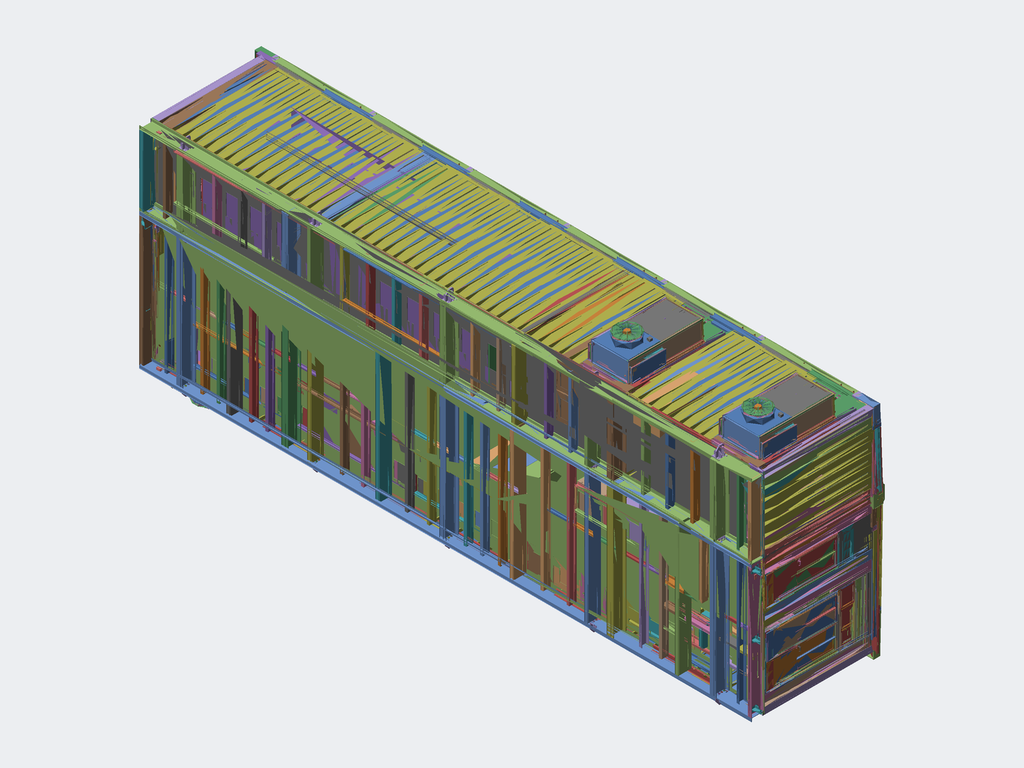Assembly | STEP file | 187 different items | 1355 placed
Parts list (item | name | quantity | parent item | size | volume):
1 | TS-BASE01_default<by machining> | x1 | in TS-BASE01 Assembly | - | 1776605339 mm3
2 | Street block | x10 | in TS-BASE01 Assembly, TS-BASE02 Assembly | 120 x 60 x 20 mm | 140702 mm3
3 | SX-lifting lug | x20 | in TS-BASE01 Assembly, TS-BASE02 Assembly | 230 x 240 x 305 mm | 3300682 mm3
4 | TS-003-01 | x12 | in TS-003 | 109.914 x 59.871 x 2995 mm | 1488875 mm3
5 | TS-003-02 | x90 | in TS-003, TS-018 | 109.897 x 56.866 x 3 mm | 12102 mm3
6 | TS-018-01 | x2 | in TS-018 | 109.914 x 59.871 x 1030 mm | 512009 mm3
7 | TS-Z001-002 | x2 | in TS-BASE01 Assembly, TS-BASE02 Assembly | 131 x 95 x 450 mm | 260117 mm3
8 | SX-Z001-01 | x12 | in TS-BASE01 Assembly, TS-BASE02 Assembly | 131 x 95 x 2995 mm | 1988432 mm3
9 | Mirror TS-Z001-002 | x2 | in TS-BASE01 Assembly, TS-BASE02 Assembly | 131 x 95 x 450 mm | 260117 mm3
10 | TS-Z001-06 | x1 | in TS-BASE01 Assembly | 131 x 95 x 2995 mm | 1974273 mm3
11 | TS-Z001-07 | x1 | in TS-BASE01 Assembly | 131 x 95 x 1203 mm | 758625 mm3
12 | Mirror TS-Z001-07 | x1 | in TS-BASE01 Assembly | 131 x 95 x 1203 mm | 758625 mm3
13 | Mirror TS-Z001-06 | x1 | in TS-BASE01 Assembly | 131 x 95 x 2995 mm | 1974273 mm3
14 | SX-platform lug | x5 | in TS-BASE01 Assembly | 170 x 218 x 196 mm | 1261021 mm3
15 | MC-Base_default<by machining> | x1 | in TS-BASE01 Assembly | 2202 x 100 x 740 mm | 7123647 mm3
16 | SW-102-Base1_default<by machining> | x1 | in TS-BASE01 Assembly | 3206 x 100 x 1155 mm | 10664759 mm3
17 | SW-102-Base2_default<by machining> | x1 | in TS-BASE01 Assembly | 3604 x 100 x 1155 mm | 11682960 mm3
18 | SW-102-Base3_default<by machining> | x1 | in TS-BASE01 Assembly | 2705 x 100 x 1155 mm | 9416033 mm3
19 | 400-TX-103_default<by machining> | x1 | in TS-BASE01 Assembly | 2050 x 1750 x 1280 mm | 1654351010 mm3
20 | 110VDC cabinet | x1 | in TS-BASE01 Assembly | 4265 x 2106 x 827 mm | 7288083743 mm3
21 | 400-MC-101 | x1 | in TS-BASE01 Assembly | 2242 x 2200 x 800 mm | 3938278879 mm3
22 | 400-SW-102 | x1 | in TS-BASE01 Assembly | 9074 x 2533 x 1310 mm | 27905066330 mm3
23 | TS-S24 | x4 | in TS-Pit-0001, TS-Pit-0002 | 3411 x 225 x 122 mm | 3346088 mm3
24 | SX-S01 | x4 | in TS-Pit-0001, TS-Pit-0002 | 3411 x 223 x 223 mm | 4765265 mm3
25 | SX-002-01 | x2 | in SX-002 | 3411 x 320 x 122 mm | 4301927 mm3
26 | Mirror SX-001-02 | x2 | in SX-002 | 3291 x 117 x 40 mm | 3023077 mm3
27 | hexagon weld nuts gb_GB_FASTENER_NUT_JSCN M8X1-N | x48 | in SX-002, SX-003, SX-001, TS-005 | 16.166 x 14 x 6.5 mm | 760.219 mm3
28 | SX-003-01 | x1 | in SX-003 | 1980 x 548 x 125 mm | 2956107 mm3
29 | SX-003-02 | x1 | in SX-003 | 120 x 98 x 1870 mm | 796406 mm3
30 | SX-003-03 | x3 | in SX-003 | 120 x 98 x 436 mm | 177136 mm3
31 | SX-003-04 | x36 | in SX-003, TS-005 | 20 x 20 x 20 mm | 5649 mm3
32 | SX-001-01 | x2 | in SX-001 | 3411 x 343 x 122 mm | 4398999 mm3
33 | SX-001-02 | x2 | in SX-001 | 3291 x 117 x 40 mm | 3023077 mm3
34 | SX-S02 | x110 | in TS-Pit-0001, TS-Pit-0002 | 3411 x 343 x 122 mm | 4146327 mm3
35 | TS-S25 TBD | x1 | in TS-Pit-0001 | 3411 x 330 x 120 mm | 4130819 mm3
36 | SX-022-01 | x2 | in SX-022 | 1870 x 122 x 78 mm | 1056252 mm3
37 | SX-022-02 | x2 | in SX-022 | 498 x 120 x 40 mm | 196950 mm3
38 | SX-022-03 | x2 | in SX-022 | 376 x 78 x 16 mm | 95014 mm3
39 | SX-022-04 | x2 | in SX-022 | 438 x 50 x 15 mm | 64937 mm3
40 | hexagon weld nuts gb_GB_FASTENER_NUT_JSCN M6-N | x114 | in SX-022, SX-004-1, TS-006 | 12.702 x 11 x 5 mm | 362.782 mm3
41 | SX-023-01 | x3 | in SX-023 | 620.667 x 418.001 x 17 mm | 629172 mm3
42 | Generic block | x72 | in SX-023, SX-018, SX-019, SX-020, SX-021, TS-007 | 16 x 15 x 16 mm | 1666 mm3
43 | TS-S93 | x1 | in SX-022 | 1870 x 502 x 1.2 mm | 1125828 mm3
44 | SX-004-01 | x3 | in SX-004-1 | 830.5 x 1503 x 122 mm | 3328995 mm3
45 | SX-004-02 | x3 | in SX-004-1 | 2341 x 159.5 x 122 mm | 2176769 mm3
46 | SX-004-03 | x3 | in SX-004-1 | 2341 x 182.5 x 122 mm | 2234839 mm3
47 | SX-004-04 | x3 | in SX-004-1 | 295.5 x 1503 x 122 mm | 1401586 mm3
48 | SX-004-05 | x6 | in SX-004-1 | 80 x 80 x 1480 mm | 692801 mm3
49 | SX-004-06 | x3 | in SX-004-1 | 80 x 80 x 2996 mm | 1398905 mm3
50 | SX-004-07 | x3 | in SX-004-1 | 78 x 30 x 2285 mm | 595601 mm3
51 | SX-004-08 | x6 | in SX-004-1 | 78 x 55 x 1157 mm | 296255 mm3
52 | SX-004-09 | x12 | in SX-004-1 | 35.36 x 28 x 2 mm | 1980 mm3
53 | SX-004-10 | x6 | in SX-004-1 | 50 x 41.5 x 1450 mm | 359516 mm3
54 | SX-004-11 | x3 | in SX-004-1 | 80 x 80 x 583 mm | 273575 mm3
55 | hexagon weld nuts gb_GB_FASTENER_NUT_JSCN M10X1.25-N | x45 | in SX-004-1 | 19.63 x 17 x 8 mm | 1354 mm3
56 | Mirror SX-004-06 | x3 | in SX-004-1 | 80 x 80 x 2996 mm | 1398905 mm3
57 | Mirror SX-004-07 | x3 | in SX-004-1 | 78 x 30 x 2285 mm | 595601 mm3
58 | SX-018-01 | x3 | in SX-018 | 733.501 x 1156 x 39 mm | 1117347 mm3
59 | SX-019-01 | x3 | in SX-019 | 553.501 x 1156 x 39 mm | 1189925 mm3
60 | SX-019-02 | x6 | in SX-019 | 890 x 276 x 115 mm | 267602 mm3
61 | SX-020-01 | x3 | in SX-020 | 251.001 x 1156 x 39 mm | 904876 mm3
62 | SX-021-01 | x3 | in SX-021 | 736.001 x 1156 x 39 mm | 2140598 mm3
63 | TS-S77 TBD | x2 | in TS-Pit-0001, TS-Pit-0002 | 3411 x 400 x 120 mm | 4608204 mm3
64 | TS-S28_DefaultSM-FLAT-PATTERN | x1 | in TS-Pit-0001 | 3411 x 262 x 122 mm | 3915643 mm3
65 | SX-006-01 | x1 | in SX-006 | 1076 x 1051 x 125 mm | 3069704 mm3
66 | SX-006-02 | x1 | in SX-006 | 120 x 98 x 965.5 mm | 412579 mm3
67 | SX-006-03 | x1 | in SX-006 | 120 x 398 x 965.5 mm | 988273 mm3
68 | SX-006-04 | x12 | in SX-006 | 16 x 16 x 16 mm | 2921 mm3
69 | TS-S57_DefaultSM-FLAT-PATTERN | x1 | in TS-Pit-0001 | 3411 x 262 x 122 mm | 3915896 mm3
70 | TS-005-01 | x1 | in TS-005 | 1780 x 548 x 125 mm | 2679291 mm3
71 | TS-005-02 | x1 | in TS-005 | 120 x 98 x 1670 mm | 710619 mm3
72 | TS-005-03 | x3 | in TS-005 | 120 x 98 x 436 mm | 177136 mm3
73 | TS-006-01 | x2 | in TS-006 | 1670 x 122 x 78 mm | 940094 mm3
74 | TS-006-02 | x2 | in TS-006 | 498 x 120 x 40 mm | 196950 mm3
75 | TS-006-03 | x2 | in TS-006 | 376 x 78 x 16 mm | 95014 mm3
76 | TS-006-04 | x2 | in TS-006 | 438 x 50 x 15 mm | 64937 mm3
77 | TS-007-01 | x3 | in TS-007 | 554 x 418.001 x 17 mm | 565980 mm3
78 | TS-S92 | x1 | in TS-006 | 1670 x 502 x 1.2 mm | 1005348 mm3
79 | TS-010-01 | x2 | in TS-010 | 120 x 100 x 572.5 mm | 586310 mm3
80 | SX-010-03 | x112 | in TS-010, SX-012, TS-019, TS-021 | 96 x 50 x 3 mm | 14400 mm3
81 | SX-012-01 | x14 | in SX-012 | 120 x 100 x 2995 mm | 3086157 mm3
82 | TS-008-01 | x2 | in TS-008 | 120 x 100 x 615 mm | 571993 mm3
83 | TS-001-02 | x4 | in TS-008 | 96 x 50 x 3 mm | 14400 mm3
84 | TS-019-01 | x8 | in TS-019 | 120 x 100 x 453 mm | 401974 mm3
85 | Mirror TS-008-011 | x2 | in Mirror TS-0081 | 120 x 100 x 615 mm | 571993 mm3
86 | Mirror TS-001-021 | x4 | in Mirror TS-0081 | 96 x 50 x 3 mm | 14400 mm3
87 | Mirror TS-019-01 | x2 | in Mirror TS-019 | 120 x 100 x 453 mm | 401974 mm3
88 | Mirror SX-010-031 | x4 | in Mirror TS-019 | 96 x 50 x 3 mm | 14400 mm3
89 | TS-S40 | x1 | in TS-Pit-0001 | 240 x 140 x 815 mm | 1340937 mm3
90 | SX-S31 | x12 | in TS-Pit-0001, TS-Pit-0002 | 240 x 140 x 2995 mm | 5007531 mm3
91 | SX-S32 | x2 | in TS-Pit-0001, TS-Pit-0002 | 240 x 140 x 450 mm | 598692 mm3
92 | TS-S79 | x2 | in TS-Pit-0001, TS-Pit-0002 | 240 x 140 x 2010 mm | 3210076 mm3
93 | Mirror SX-S32 | x2 | in TS-Pit-0001, TS-Pit-0002 | 240 x 140 x 450 mm | 598692 mm3
94 | Mirror TS-S79 | x2 | in TS-Pit-0001, TS-Pit-0002 | 240 x 140 x 2010 mm | 3210076 mm3
95 | Mirror TS-S40 | x1 | in TS-Pit-0001 | 240 x 140 x 815 mm | 1340937 mm3
96 | SX-S36 | x20 | in TS-Pit-0001, TS-Pit-0002 | 200 x 140 x 2 mm | 55817 mm3
97 | TS-S80 | x1 | in TS-Pit-0001 | 4045 x 380 x 97 mm | 5054054 mm3
98 | TS-S44 | x47 | in TS-Pit-0001 | 4045 x 403 x 100 mm | 5175456 mm3
99 | TS-S81 | x1 | in TS-Pit-0001 | 4045 x 393 x 100 mm | 5094556 mm3
100 | SX-014-01 | x12 | in SX-014 | 134 x 49.886 x 2995 mm | 1979829 mm3
101 | SX-013-02 | x54 | in SX-014, TS-020 | 104.087 x 50 x 3 mm | 15613 mm3
102 | TS-S47 | x48 | in TS-Pit-0001 | 4250 x 403 x 62 mm | 4791334 mm3
103 | TS-S34 | x1 | in TS-Pit-0001 | 561 x 33 x 3283 mm | 1948503 mm3
104 | SX-S26 | x1 | in TS-Pit-0001 | 1865 x 502.5 x 30 mm | 1150989 mm3
105 | TS-S35 | x1 | in TS-Pit-0001 | 398 x 4.2 x 3283 mm | 1369495 mm3
106 | SX-S18 | x29 | in TS-Pit-0001, TS-Pit-0002 | 978 x 4.2 x 3283 mm | 3879324 mm3
107 | TS-S36 | x1 | in TS-Pit-0001 | 408.999 x 97.999 x 3283 mm | 1985800 mm3
108 | SX-S22 | x3 | in TS-Pit-0001, TS-Pit-0002 | 1498 x 785 x 1.2 mm | 1410637 mm3
109 | SX-S20 | x3 | in TS-Pit-0001, TS-Pit-0002 | 2285 x 159.5 x 1.2 mm | 436964 mm3
110 | SX-S21 | x3 | in TS-Pit-0001, TS-Pit-0002 | 2285 x 177.5 x 1.2 mm | 486320 mm3
111 | SX-S23 | x3 | in TS-Pit-0001, TS-Pit-0002 | 1498 x 213 x 1.2 mm | 382614 mm3
112 | TS-S32 | x1 | in TS-Pit-0001 | 95.999 x 457.999 x 3283 mm | 1963337 mm3
113 | TS-S33 | x1 | in TS-Pit-0001 | 1665 x 502.5 x 30 mm | 1030433 mm3
114 | TS-S31 | x1 | in TS-Pit-0001 | 702 x 4.2 x 3283 mm | 2405331 mm3
115 | SX-S19 | x1 | in TS-Pit-0001 | 961 x 1005 x 30 mm | 1216636 mm3
116 | TS-S82 | x1 | in TS-Pit-0001 | 3411 x 303 x 122 mm | 3873447 mm3
117 | SX-S16 | x4 | in TS-Pit-0001, TS-Pit-0002 | 658 x 4.2 x 3283 mm | 2609753 mm3
118 | TS-S83 | x1 | in TS-Pit-0001 | 720 x 3283 x 43 mm | 3005343 mm3
119 | TS-S84 | x1 | in TS-Pit-0001 | 800 x 3283 x 43 mm | 3320511 mm3
120 | TS-S85 | x1 | in TS-Pit-0001 | 528 x 3283 x 43 mm | 2240757 mm3
121 | TS-S86 | x1 | in TS-Pit-0001 | 488 x 3283 x 43 mm | 2083173 mm3
122 | TS-S87 TBD | x2 | in TS-Pit-0001, TS-Pit-0002 | 402 x 4.3 x 3283 mm | 1592924 mm3
123 | TS-S88 | x1 | in TS-Pit-0001 | 503 x 33 x 3283 mm | 1756521 mm3
124 | TS-020-01 | x2 | in TS-020 | 134 x 49.886 x 1030 mm | 673543 mm3
125 | TS-S90 | x1 | in TS-Pit-0001 | 4250 x 403 x 62 mm | 4816834 mm3
126 | TS-S89 | x1 | in TS-Pit-0001 | 4250 x 380 x 62 mm | 4689334 mm3
127 | TS-S53 | x1 | in TS-Pit-0001 | 2995 x 298.377 x 60 mm | 2109135 mm3
128 | TS-S51 | x1 | in TS-Pit-0001 | 1320 x 231.983 x 555 mm | 1200931 mm3
129 | TS-S50 | x6 | in TS-Pit-0001 | 150.007 x 206.045 x 2995 mm | 2202698 mm3
130 | Mirror TS-S53 | x1 | in TS-Pit-0001 | 2995 x 298.377 x 60 mm | 2109135 mm3
131 | TS-S54 | x1 | in TS-Pit-0001 | 200.554 x 238.201 x 100 mm | 167109 mm3
132 | TS-S55 | x7 | in TS-Pit-0001 | 102 x 207.828 x 200 mm | 142020 mm3
133 | Mirror TS-S54 | x1 | in TS-Pit-0001 | 200.554 x 238.201 x 100 mm | 167109 mm3
134 | Mirror TS-S511 | x1 | in TS-Pit-0001 | 1320 x 231.983 x 555 mm | 1200931 mm3
135 | Single door assembly | x1 | in TS-Pit-0001 | - | -
136 | 1600 door assembly | x1 | in TS-Pit-0001 | - | -
137 | 1800 door assembly | x1 | in TS-Pit-0001 | - | -
138 | MAK air conditioner | x3 | in TS-Pit-0001, TS-Pit-0002 | - | -
139 | TS-BASE02_default<by machining> | x1 | in TS-BASE02 Assembly | 19000 x 4000 x 2295 mm | 1123483782 mm3
140 | TS-Z001-001 | x1 | in TS-BASE02 Assembly | 131 x 95 x 2298 mm | 1471322 mm3
141 | Mirror TS-Z001-001 | x1 | in TS-BASE02 Assembly | 131 x 95 x 2298 mm | 1471322 mm3
142 | SW-101-Base1_default<by machining> | x1 | in TS-BASE02 Assembly | 5206 x 100 x 1440 mm | 16389310 mm3
143 | SW-101-Base2_default<by machining> | x1 | in TS-BASE02 Assembly | 5206 x 100 x 1440 mm | 16389310 mm3
144 | 400-SW-101 | x1 | in TS-BASE02 Assembly | 8870 x 2733 x 1700 mm | 38224266392 mm3
145 | PLC cabinet | x2 | in TS-BASE02 Assembly | 806 x 2100 x 805 mm | 1358956656 mm3
146 | Power distribution cabinet | x1 | in TS-BASE02 Assembly | 800 x 2100 x 550 mm | 917054924 mm3
147 | Air conditioner cabinet | x1 | in TS-BASE02 Assembly | 500 x 1900 x 550 mm | 519606146 mm3
148 | Tool cabinet | x1 | in TS-BASE02 Assembly | 800 x 1800 x 500 mm | 719981469 mm3
149 | TS-S94 | x1 | in TS-Pit-0002 | 3411 x 423 x 122 mm | 4691933 mm3
150 | TS-S95 TBD | x2 | in TS-Pit-0002 | 3411 x 300 x 120 mm | 3926160 mm3
151 | TS-021-01 | x2 | in TS-021 | 120 x 100 x 1668 mm | 1716670 mm3
152 | TS-S96 | x1 | in TS-Pit-0002 | 199 x 33 x 3283 mm | 719864 mm3
153 | Mirror TS-S96 | x1 | in TS-Pit-0002 | - | -
154 | TS-S97 TBD | x1 | in TS-Pit-0002 | 375.999 x 97.999 x 3283 mm | 1855793 mm3
155 | Mirror TS-S97 TBD | x1 | in TS-Pit-0002 | 375.999 x 97.999 x 3283 mm | 1855793 mm3
156 | TS-S98 | x1 | in TS-Pit-0002 | 790 x 3283 x 43 mm | 3281115 mm3
157 | TS-S99 | x1 | in TS-Pit-0002 | 830 x 3283 x 43 mm | 3438699 mm3
158 | TS-S100 | x1 | in TS-Pit-0002 | 498 x 3283 x 43 mm | 2122569 mm3
159 | TS-S101 | x1 | in TS-Pit-0002 | 859 x 3283 x 43 mm | 3553710 mm3
160 | TS-S13 | x1 | in TS-Pit-0002 | 2145 x 370 x 97 mm | 2636955 mm3
161 | TS-S102 | x1 | in TS-Pit-0002 | 240 x 140 x 1910 mm | 3171467 mm3
162 | Mirror TS-S102 | x1 | in TS-Pit-0002 | 240 x 140 x 1910 mm | 3171467 mm3
163 | TS-S14 | x48 | in TS-Pit-0002 | 2145 x 403 x 100 mm | 2744257 mm3
164 | TS-S15 | x1 | in TS-Pit-0002 | 2350 x 380 x 62 mm | 2592719 mm3
165 | TS-S16 | x48 | in TS-Pit-0002 | 2350 x 403 x 62 mm | 2649119 mm3
166 | TS-S20 | x1 | in TS-Pit-0002 | - | -
167 | TS-S18 | x1 | in TS-Pit-0002 | 515.803 x 221.885 x 555 mm | 694514 mm3
168 | TS-S19 | x6 | in TS-Pit-0002 | 149.959 x 207.22 x 2995 mm | 2193923 mm3
169 | TS-S17 | x1 | in TS-Pit-0002 | 1915 x 298.7 x 60 mm | 1317864 mm3
170 | TS-S23 | x7 | in TS-Pit-0002 | 122 x 207.205 x 200 mm | 149406 mm3
171 | Mirror TS-S17 | x1 | in TS-Pit-0002 | 1915 x 298.7 x 60 mm | 1317864 mm3
172 | TS-S22 | x1 | in TS-Pit-0002 | 201.003 x 230.402 x 100 mm | 163289 mm3
173 | Mirror TS-S22 | x1 | in TS-Pit-0002 | 201.003 x 230.402 x 100 mm | 163289 mm3
174 | Mirror TS-S18 | x1 | in TS-Pit-0002 | 515.803 x 221.885 x 555 mm | 694514 mm3
175 | Assembly TS-S02 | x6 | - | 590.266 x 52.135 x 120 mm | 150616 mm3
176 | Assembly TS-001-01 | x1 | in Assembly TS-001 | 590.5 x 344 x 100 mm | 582857 mm3
177 | Assembly TS-001-02 | x1 | in Assembly TS-001 | 92.488 x 46.409 x 97 mm | 21261 mm3
178 | Assembly TS-001-03 | x1 | in Assembly TS-001 | 96.717 x 50.15 x 97 mm | 22295 mm3
179 | Assembly TS-S03 | x2 | - | 120 x 3256 x 2 mm | 777120 mm3
180 | Assembly TS-S04 | x1 | - | 55 x 3256 x 90 mm | 923542 mm3
181 | Assembly TS-S06 | x1 | - | 151.963 x 210.044 x 400 mm | 364106 mm3
182 | Assembly TS-S07 | x1 | - | 100 x 140 x 100 mm | 55113 mm3
183 | Assembly TS-S01 | x6 | - | 590.109 x 52.135 x 2995 mm | 3761784 mm3
184 | Mirror assembly TS-001-01 | x1 | in Mirror assembly TS-001 | 590.5 x 344 x 100 mm | 582857 mm3
185 | Mirror assembly TS-001-02 | x1 | in Mirror assembly TS-001 | 92.488 x 46.409 x 97 mm | 21261 mm3
186 | Mirror assembly TS-001-03 | x1 | in Mirror assembly TS-001 | 96.717 x 50.15 x 97 mm | 22295 mm3
187 | Assembly TS-S09 | x1 | - | 590.109 x 52.135 x 1030 mm | 1293599 mm3
Placements (level | parent | child | x y z in mm | rotation matrix by rows), first 321 of 1451 lines:
1 | subassembly 2 | TS-Pit-0001 | -2561.957 -160.016 -20522.75 | 1 0 0 0 1 0 0 0 1
2 | TS-Pit-0001 | TS-BASE01 Assembly | -1486.871 -103.945 -616.75 | 1 0 0 0 1 0 0 0 1
3 | TS-BASE01 Assembly | TS-BASE01_default<by machining> | 1365.177 -1695.191 19655.0 | 1 0 0 0 1 0 0 0 1
3 | TS-BASE01 Assembly | Street block | -7659.823 -1895.191 17647.0 | -1 0 0 0 1 0 0 0 -1
3 | TS-BASE01 Assembly | Street block | -7980.323 -1895.191 21542.5 | 0 0 -1 0 1 0 1 0 -0
3 | TS-BASE01 Assembly | Street block | 10390.177 -1895.191 17647.0 | -1 0 0 0 1 0 0 0 -1
3 | TS-BASE01 Assembly | Street block | 10710.677 -1895.191 21292.5 | 0 0 1 0 1 0 -1 0 -0
3 | TS-BASE01 Assembly | SX-lifting lug | -6824.823 -1895.191 21752.5 | 1 0 0 0 1 0 0 0 1
3 | TS-BASE01 Assembly | SX-lifting lug | -6824.823 -1895.191 17647.0 | -1 0 0 0 1 0 0 0 -1
3 | TS-BASE01 Assembly | SX-lifting lug | -2784.823 -1895.191 21752.5 | 1 0 0 0 1 0 0 0 1
3 | TS-BASE01 Assembly | SX-lifting lug | -2784.823 -1895.191 17647.0 | -1 0 0 0 1 0 0 0 -1
3 | TS-BASE01 Assembly | SX-lifting lug | 1285.177 -1895.191 17647.0 | -1 0 0 0 1 0 0 0 -1
3 | TS-BASE01 Assembly | SX-lifting lug | 1285.177 -1895.191 21752.5 | 1 0 0 0 1 0 0 0 1
3 | TS-BASE01 Assembly | SX-lifting lug | 5755.177 -1895.191 21752.5 | 1 0 0 0 1 0 0 0 1
3 | TS-BASE01 Assembly | SX-lifting lug | 5755.177 -1895.191 17647.0 | -1 0 0 0 1 0 0 0 -1
3 | TS-BASE01 Assembly | SX-lifting lug | 9620.177 -1895.191 17647.0 | -1 0 0 0 1 0 0 0 -1
3 | TS-BASE01 Assembly | SX-lifting lug | 9620.177 -1895.191 21752.5 | 1 0 0 0 1 0 0 0 1
3 | TS-BASE01 Assembly | TS-003 | 6375.177 1771.711 21668.782 | 0 0 1 0 1 0 -1 0 0
4 | TS-003 | TS-003-01 | 3890.909 -3059.221 1495.0 | 1 0 0 0 1 0 0 0 1
4 | TS-003 | TS-003-02 | 4272.867 -3750.281 4490.0 | 1 0 0 0 1 0 0 0 1
4 | TS-003 | TS-003-02 | 4272.867 -3750.281 3991.33 | 1 0 0 0 1 0 0 0 1
4 | TS-003 | TS-003-02 | 4272.867 -3750.281 3492.66 | 1 0 0 0 1 0 0 0 1
4 | TS-003 | TS-003-02 | 4272.867 -3750.281 2993.99 | 1 0 0 0 1 0 0 0 1
4 | TS-003 | TS-003-02 | 4272.867 -3750.281 2495.32 | 1 0 0 0 1 0 0 0 1
4 | TS-003 | TS-003-02 | 4272.867 -3750.281 1996.65 | 1 0 0 0 1 0 0 0 1
4 | TS-003 | TS-003-02 | 4272.867 -3750.281 1497.98 | 1 0 0 0 1 0 0 0 1
3 | TS-BASE01 Assembly | TS-003 | 3380.177 1771.711 21668.782 | 0 0 1 0 1 0 -1 0 0
4 | TS-003 | TS-003-01 | 3890.909 -3059.221 1495.0 | 1 0 0 0 1 0 0 0 1
4 | TS-003 | TS-003-02 | 4272.867 -3750.281 4490.0 | 1 0 0 0 1 0 0 0 1
4 | TS-003 | TS-003-02 | 4272.867 -3750.281 3991.33 | 1 0 0 0 1 0 0 0 1
4 | TS-003 | TS-003-02 | 4272.867 -3750.281 3492.66 | 1 0 0 0 1 0 0 0 1
4 | TS-003 | TS-003-02 | 4272.867 -3750.281 2993.99 | 1 0 0 0 1 0 0 0 1
4 | TS-003 | TS-003-02 | 4272.867 -3750.281 2495.32 | 1 0 0 0 1 0 0 0 1
4 | TS-003 | TS-003-02 | 4272.867 -3750.281 1996.65 | 1 0 0 0 1 0 0 0 1
4 | TS-003 | TS-003-02 | 4272.867 -3750.281 1497.98 | 1 0 0 0 1 0 0 0 1
3 | TS-BASE01 Assembly | TS-003 | 385.177 1771.711 21668.782 | 0 0 1 0 1 0 -1 0 0
4 | TS-003 | TS-003-01 | 3890.909 -3059.221 1495.0 | 1 0 0 0 1 0 0 0 1
4 | TS-003 | TS-003-02 | 4272.867 -3750.281 4490.0 | 1 0 0 0 1 0 0 0 1
4 | TS-003 | TS-003-02 | 4272.867 -3750.281 3991.33 | 1 0 0 0 1 0 0 0 1
4 | TS-003 | TS-003-02 | 4272.867 -3750.281 3492.66 | 1 0 0 0 1 0 0 0 1
4 | TS-003 | TS-003-02 | 4272.867 -3750.281 2993.99 | 1 0 0 0 1 0 0 0 1
4 | TS-003 | TS-003-02 | 4272.867 -3750.281 2495.32 | 1 0 0 0 1 0 0 0 1
4 | TS-003 | TS-003-02 | 4272.867 -3750.281 1996.65 | 1 0 0 0 1 0 0 0 1
4 | TS-003 | TS-003-02 | 4272.867 -3750.281 1497.98 | 1 0 0 0 1 0 0 0 1
3 | TS-BASE01 Assembly | TS-003 | -2609.823 1771.711 21668.782 | 0 0 1 0 1 0 -1 0 0
4 | TS-003 | TS-003-01 | 3890.909 -3059.221 1495.0 | 1 0 0 0 1 0 0 0 1
4 | TS-003 | TS-003-02 | 4272.867 -3750.281 4490.0 | 1 0 0 0 1 0 0 0 1
4 | TS-003 | TS-003-02 | 4272.867 -3750.281 3991.33 | 1 0 0 0 1 0 0 0 1
4 | TS-003 | TS-003-02 | 4272.867 -3750.281 3492.66 | 1 0 0 0 1 0 0 0 1
4 | TS-003 | TS-003-02 | 4272.867 -3750.281 2993.99 | 1 0 0 0 1 0 0 0 1
4 | TS-003 | TS-003-02 | 4272.867 -3750.281 2495.32 | 1 0 0 0 1 0 0 0 1
4 | TS-003 | TS-003-02 | 4272.867 -3750.281 1996.65 | 1 0 0 0 1 0 0 0 1
4 | TS-003 | TS-003-02 | 4272.867 -3750.281 1497.98 | 1 0 0 0 1 0 0 0 1
3 | TS-BASE01 Assembly | TS-003 | -5604.823 1771.711 21668.782 | 0 0 1 0 1 0 -1 0 0
4 | TS-003 | TS-003-01 | 3890.909 -3059.221 1495.0 | 1 0 0 0 1 0 0 0 1
4 | TS-003 | TS-003-02 | 4272.867 -3750.281 4490.0 | 1 0 0 0 1 0 0 0 1
4 | TS-003 | TS-003-02 | 4272.867 -3750.281 3991.33 | 1 0 0 0 1 0 0 0 1
4 | TS-003 | TS-003-02 | 4272.867 -3750.281 3492.66 | 1 0 0 0 1 0 0 0 1
4 | TS-003 | TS-003-02 | 4272.867 -3750.281 2993.99 | 1 0 0 0 1 0 0 0 1
4 | TS-003 | TS-003-02 | 4272.867 -3750.281 2495.32 | 1 0 0 0 1 0 0 0 1
4 | TS-003 | TS-003-02 | 4272.867 -3750.281 1996.65 | 1 0 0 0 1 0 0 0 1
4 | TS-003 | TS-003-02 | 4272.867 -3750.281 1497.98 | 1 0 0 0 1 0 0 0 1
3 | TS-BASE01 Assembly | TS-003 | -8599.823 1771.711 21668.782 | 0 0 1 0 1 0 -1 0 0
4 | TS-003 | TS-003-01 | 3890.909 -3059.221 1495.0 | 1 0 0 0 1 0 0 0 1
4 | TS-003 | TS-003-02 | 4272.867 -3750.281 4490.0 | 1 0 0 0 1 0 0 0 1
4 | TS-003 | TS-003-02 | 4272.867 -3750.281 3991.33 | 1 0 0 0 1 0 0 0 1
4 | TS-003 | TS-003-02 | 4272.867 -3750.281 3492.66 | 1 0 0 0 1 0 0 0 1
4 | TS-003 | TS-003-02 | 4272.867 -3750.281 2993.99 | 1 0 0 0 1 0 0 0 1
4 | TS-003 | TS-003-02 | 4272.867 -3750.281 2495.32 | 1 0 0 0 1 0 0 0 1
4 | TS-003 | TS-003-02 | 4272.867 -3750.281 1996.65 | 1 0 0 0 1 0 0 0 1
4 | TS-003 | TS-003-02 | 4272.867 -3750.281 1497.98 | 1 0 0 0 1 0 0 0 1
3 | TS-BASE01 Assembly | TS-018 | -9629.823 1771.711 21668.782 | 0 0 1 0 1 0 -1 0 0
4 | TS-018 | TS-018-01 | 3890.909 -3059.221 1495.0 | 1 0 0 0 1 0 0 0 1
4 | TS-018 | TS-003-02 | 4272.867 -3750.281 2525.0 | 1 0 0 0 1 0 0 0 1
4 | TS-018 | TS-003-02 | 4272.867 -3750.281 2011.5 | 1 0 0 0 1 0 0 0 1
4 | TS-018 | TS-003-02 | 4272.867 -3750.281 1498.0 | 1 0 0 0 1 0 0 0 1
3 | TS-BASE01 Assembly | TS-Z001-002 | 10800.177 -1744.191 17554.5 | 0 0 -1 0 1 0 1 0 0
3 | TS-BASE01 Assembly | SX-Z001-01 | 10350.177 -1744.191 17554.5 | 0 0 -1 0 1 0 1 0 0
3 | TS-BASE01 Assembly | SX-Z001-01 | 7355.177 -1744.191 17554.5 | 0 0 -1 0 1 0 1 0 0
3 | TS-BASE01 Assembly | SX-Z001-01 | 4360.177 -1744.191 17554.5 | 0 0 -1 0 1 0 1 0 0
3 | TS-BASE01 Assembly | SX-Z001-01 | 1365.177 -1744.191 17554.5 | 0 0 -1 0 1 0 1 0 0
3 | TS-BASE01 Assembly | SX-Z001-01 | -1629.823 -1744.191 17554.5 | 0 0 -1 0 1 0 1 0 0
3 | TS-BASE01 Assembly | SX-Z001-01 | -4624.823 -1744.191 17554.5 | 0 0 -1 0 1 0 1 0 0
3 | TS-BASE01 Assembly | Mirror TS-Z001-002 | -8069.823 -1744.191 17554.5 | 0 0 -1 0 1 0 1 0 0
3 | TS-BASE01 Assembly | TS-Z001-06 | -8072.823 -1744.191 18757.5 | 1 0 0 0 1 0 0 0 1
3 | TS-BASE01 Assembly | TS-Z001-07 | -8072.823 -1744.191 17557.5 | 1 0 0 0 1 0 0 0 1
3 | TS-BASE01 Assembly | Mirror TS-Z001-07 | 10803.177 -1744.191 17557.5 | -1 0 0 0 1 0 0 0 -1
3 | TS-BASE01 Assembly | Mirror TS-Z001-06 | 10803.177 -1744.191 18757.5 | -1 0 0 0 1 0 0 0 -1
3 | TS-BASE01 Assembly | SX-platform lug | 10710.677 -1904.191 21502.5 | 0 0 1 0 1 0 -1 0 -0
3 | TS-BASE01 Assembly | SX-platform lug | -7980.323 -1904.191 21352.5 | 0 0 -1 0 1 0 1 0 -0
3 | TS-BASE01 Assembly | SX-platform lug | -7980.323 -1904.191 19152.5 | 0 0 -1 0 1 0 1 0 -0
3 | TS-BASE01 Assembly | SX-platform lug | 10710.677 -1904.191 19652.5 | 0 0 1 0 1 0 -1 0 -0
3 | TS-BASE01 Assembly | SX-platform lug | 10710.677 -1904.191 17802.5 | 0 0 1 0 1 0 -1 0 -0
3 | TS-BASE01 Assembly | Street block | -7659.823 -1895.191 17659.5 | 1 0 0 0 1 0 0 0 1
3 | TS-BASE01 Assembly | MC-Base_default<by machining> | 6041.177 -1689.191 20404.5 | 1 0 0 0 1 0 0 0 1
3 | TS-BASE01 Assembly | SW-102-Base1_default<by machining> | -5216.823 -1689.191 18600.5 | 1 0 0 0 1 0 0 0 1
3 | TS-BASE01 Assembly | SW-102-Base2_default<by machining> | -1811.823 -1689.191 18600.5 | 1 0 0 0 1 0 0 0 1
3 | TS-BASE01 Assembly | SW-102-Base3_default<by machining> | 1342.677 -1689.191 18600.5 | -1 0 0 0 1 0 0 0 -1
3 | TS-BASE01 Assembly | 400-TX-103_default<by machining> | 9035.177 -1689.191 18827.5 | 1 0 0 0 1 0 0 0 1
3 | TS-BASE01 Assembly | 110VDC cabinet | 3910.177 -1689.191 18177.5 | 1 0 0 0 1 0 0 0 1
3 | TS-BASE01 Assembly | 400-MC-101 | 5941.177 -1589.191 20404.5 | 1 0 0 0 1 0 0 0 1
3 | TS-BASE01 Assembly | 400-SW-102 | -6318.823 -1589.191 17962.5 | 1 0 0 0 1 0 0 0 1
2 | TS-Pit-0001 | TS-S24 | -9559.694 -1850.136 20935.75 | 0 0 1 1 0 0 0 1 0
2 | TS-Pit-0001 | SX-S01 | -9361.694 -1850.136 16937.75 | 0 -1 0 1 0 0 0 0 1
2 | TS-Pit-0001 | SX-S01 | 9316.306 -1850.136 17135.75 | 0 0 -1 1 0 0 0 -1 0
2 | TS-Pit-0001 | SX-002 | -12891.694 48.765 20728.153 | 0 0 1 1 0 0 0 1 -0
3 | SX-002 | SX-002-01 | -1898.901 -112.403 3332.0 | 1 0 0 0 1 0 0 0 1
3 | SX-002 | Mirror SX-001-02 | 1512.099 -110.403 3332.0 | 1 0 0 0 0 1 0 -1 0
3 | SX-002 | hexagon weld nuts gb_GB_FASTENER_NUT_JSCN M8X1-N | 913.099 -99.303 3366.0 | 1 0 0 0 0 1 0 -1 -0
3 | SX-002 | hexagon weld nuts gb_GB_FASTENER_NUT_JSCN M8X1-N | 712.099 -99.303 3366.0 | 1 0 0 0 0 1 0 -1 -0
3 | SX-002 | hexagon weld nuts gb_GB_FASTENER_NUT_JSCN M8X1-N | 511.099 -99.303 3366.0 | 1 0 0 0 0 1 0 -1 -0
3 | SX-002 | hexagon weld nuts gb_GB_FASTENER_NUT_JSCN M8X1-N | 913.099 -99.303 3426.0 | 1 0 0 0 0 1 0 -1 -0
3 | SX-002 | hexagon weld nuts gb_GB_FASTENER_NUT_JSCN M8X1-N | 712.099 -99.303 3426.0 | 1 0 0 0 0 1 0 -1 -0
3 | SX-002 | hexagon weld nuts gb_GB_FASTENER_NUT_JSCN M8X1-N | 511.099 -99.303 3426.0 | 1 0 0 0 0 1 0 -1 -0
2 | TS-Pit-0001 | SX-003 | -9499.197 1208.266 19793.565 | 0 0 -1 0 1 0 1 0 0
3 | SX-003 | SX-003-01 | -1047.815 -195.402 62.498 | 1 0 0 0 1 0 0 0 1
3 | SX-003 | SX-003-02 | -1045.565 242.598 60.498 | 0 0 1 0 1 0 -1 0 0
3 | SX-003 | SX-003-03 | 402.185 -180.402 60.498 | 0 -1 0 0 0 1 -1 0 -0
3 | SX-003 | SX-003-03 | -135.815 -180.402 60.498 | 0 -1 0 0 0 1 -1 0 -0
3 | SX-003 | SX-003-03 | -673.815 -180.402 60.498 | 0 -1 0 0 0 1 -1 0 -0
3 | SX-003 | hexagon weld nuts gb_GB_FASTENER_NUT_JSCN M8X1-N | 764.185 -186.902 36.498 | 1 0 0 0 0 1 0 -1 -0
3 | SX-003 | hexagon weld nuts gb_GB_FASTENER_NUT_JSCN M8X1-N | 764.185 -186.902 -33.502 | 1 0 0 0 0 1 0 -1 -0
3 | SX-003 | hexagon weld nuts gb_GB_FASTENER_NUT_JSCN M8X1-N | 413.385 -186.902 36.498 | 1 0 0 0 0 1 0 -1 -0
3 | SX-003 | hexagon weld nuts gb_GB_FASTENER_NUT_JSCN M8X1-N | 413.385 -186.902 -33.502 | 1 0 0 0 0 1 0 -1 -0
3 | SX-003 | hexagon weld nuts gb_GB_FASTENER_NUT_JSCN M8X1-N | 62.585 -186.902 36.498 | 1 0 0 0 0 1 0 -1 -0
3 | SX-003 | hexagon weld nuts gb_GB_FASTENER_NUT_JSCN M8X1-N | 62.585 -186.902 -33.502 | 1 0 0 0 0 1 0 -1 -0
3 | SX-003 | hexagon weld nuts gb_GB_FASTENER_NUT_JSCN M8X1-N | -288.215 -186.902 36.498 | 1 0 0 0 0 1 0 -1 -0
3 | SX-003 | hexagon weld nuts gb_GB_FASTENER_NUT_JSCN M8X1-N | -288.215 -186.902 -33.502 | 1 0 0 0 0 1 0 -1 -0
3 | SX-003 | hexagon weld nuts gb_GB_FASTENER_NUT_JSCN M8X1-N | -639.015 -186.902 36.498 | 1 0 0 0 0 1 0 -1 -0
3 | SX-003 | hexagon weld nuts gb_GB_FASTENER_NUT_JSCN M8X1-N | -639.015 -186.902 -33.502 | 1 0 0 0 0 1 0 -1 -0
3 | SX-003 | hexagon weld nuts gb_GB_FASTENER_NUT_JSCN M8X1-N | -989.815 -186.902 36.498 | 1 0 0 0 0 1 0 -1 -0
3 | SX-003 | hexagon weld nuts gb_GB_FASTENER_NUT_JSCN M8X1-N | -989.815 -186.902 -33.502 | 1 0 0 0 0 1 0 -1 -0
3 | SX-003 | SX-003-04 | 787.185 -145.402 60.498 | -0.9237 -0.383 0 -0.383 0.9237 0 0 0 -1
3 | SX-003 | SX-003-04 | 787.185 -45.402 60.498 | -0.9237 -0.383 0 -0.383 0.9237 0 0 0 -1
3 | SX-003 | SX-003-04 | 787.185 54.598 60.498 | -0.9237 -0.383 0 -0.383 0.9237 0 0 0 -1
3 | SX-003 | SX-003-04 | 427.185 -145.402 60.498 | -0.9237 -0.383 0 -0.383 0.9237 0 0 0 -1
3 | SX-003 | SX-003-04 | 427.185 -45.402 60.498 | -0.9237 -0.383 0 -0.383 0.9237 0 0 0 -1
3 | SX-003 | SX-003-04 | 427.185 54.598 60.498 | -0.9237 -0.383 0 -0.383 0.9237 0 0 0 -1
3 | SX-003 | SX-003-04 | 67.185 -145.402 60.498 | -0.9237 -0.383 0 -0.383 0.9237 0 0 0 -1
3 | SX-003 | SX-003-04 | 67.185 -45.402 60.498 | -0.9237 -0.383 0 -0.383 0.9237 0 0 0 -1
3 | SX-003 | SX-003-04 | 67.185 54.598 60.498 | -0.9237 -0.383 0 -0.383 0.9237 0 0 0 -1
3 | SX-003 | SX-003-04 | -292.815 -145.402 60.498 | -0.9237 -0.383 0 -0.383 0.9237 0 0 0 -1
3 | SX-003 | SX-003-04 | -292.815 -45.402 60.498 | -0.9237 -0.383 0 -0.383 0.9237 0 0 0 -1
3 | SX-003 | SX-003-04 | -292.815 54.598 60.498 | -0.9237 -0.383 0 -0.383 0.9237 0 0 0 -1
3 | SX-003 | SX-003-04 | -652.815 -145.402 60.498 | -0.9237 -0.383 0 -0.383 0.9237 0 0 0 -1
3 | SX-003 | SX-003-04 | -652.815 -45.402 60.498 | -0.9237 -0.383 0 -0.383 0.9237 0 0 0 -1
3 | SX-003 | SX-003-04 | -652.815 54.598 60.498 | -0.9237 -0.383 0 -0.383 0.9237 0 0 0 -1
3 | SX-003 | SX-003-04 | -1012.815 -145.402 60.498 | -0.9237 -0.383 0 -0.383 0.9237 0 0 0 -1
3 | SX-003 | SX-003-04 | -1012.815 -45.402 60.498 | -0.9237 -0.383 0 -0.383 0.9237 0 0 0 -1
3 | SX-003 | SX-003-04 | -1012.815 54.598 60.498 | -0.9237 -0.383 0 -0.383 0.9237 0 0 0 -1
2 | TS-Pit-0001 | SX-001 | -9559.694 1560.864 18745.75 | 0 0 1 -1 0 0 0 -1 -0
3 | SX-001 | SX-001-01 | -0.0 -0.0 -0.0 | 1 0 0 0 1 0 0 0 1
3 | SX-001 | SX-001-02 | 0.0 2.0 -0.0 | -1 0 0 0 0 -1 0 -1 -0
3 | SX-001 | hexagon weld nuts gb_GB_FASTENER_NUT_JSCN M8X1-N | 599.0 13.5 34.0 | 1 0 0 0 0 1 0 -1 0
3 | SX-001 | hexagon weld nuts gb_GB_FASTENER_NUT_JSCN M8X1-N | 599.0 13.5 94.0 | 1 0 0 0 0 1 0 -1 0
3 | SX-001 | hexagon weld nuts gb_GB_FASTENER_NUT_JSCN M8X1-N | 800.0 13.5 34.0 | 1 0 0 0 0 1 0 -1 0
3 | SX-001 | hexagon weld nuts gb_GB_FASTENER_NUT_JSCN M8X1-N | 800.0 13.5 94.0 | 1 0 0 0 0 1 0 -1 0
3 | SX-001 | hexagon weld nuts gb_GB_FASTENER_NUT_JSCN M8X1-N | 1001.0 13.5 34.0 | 1 0 0 0 0 1 0 -1 0
3 | SX-001 | hexagon weld nuts gb_GB_FASTENER_NUT_JSCN M8X1-N | 1001.0 13.5 94.0 | 1 0 0 0 0 1 0 -1 0
2 | TS-Pit-0001 | SX-S02 | -9559.694 -1850.136 18105.75 | 0 0 1 1 0 0 0 1 -0
2 | TS-Pit-0001 | SX-S02 | -9559.694 -1850.136 17785.75 | 0 0 1 1 0 0 0 1 -0
2 | TS-Pit-0001 | SX-S02 | -9559.694 -1850.136 17465.75 | 0 0 1 1 0 0 0 1 -0
2 | TS-Pit-0001 | TS-S25 TBD | -9559.694 1560.864 17465.75 | 0 0 1 -1 0 0 0 -1 0
2 | TS-Pit-0001 | SX-022 | -9496.186 1070.864 20296.197 | 0 1 0 0 0 -1 -1 0 0
3 | SX-022 | SX-022-01 | -359.553 -47.508 522.0 | 1 0 0 0 1 0 0 0 1
3 | SX-022 | SX-022-01 | 1590.447 -47.508 96.0 | -1 0 0 0 1 0 0 0 -1
3 | SX-022 | SX-022-02 | -319.553 -45.508 60.0 | 0 0 -1 0 1 0 1 0 -0
3 | SX-022 | SX-022-02 | 1550.447 -45.508 558.0 | 0 0 1 0 1 0 -1 0 0
3 | SX-022 | SX-022-03 | 265.114 -47.508 497.0 | 0 1 0 0 0 -1 -1 0 -0
3 | SX-022 | SX-022-03 | 887.781 -47.508 497.0 | 0 1 0 0 0 -1 -1 0 -0
3 | SX-022 | SX-022-04 | 951.781 54.492 90.0 | 0 -1 0 0 0 -1 1 0 -0
3 | SX-022 | SX-022-04 | 329.114 54.492 90.0 | 0 -1 0 0 0 -1 1 0 -0
3 | SX-022 | hexagon weld nuts gb_GB_FASTENER_NUT_JSCN M6-N | 1500.447 -58.508 540.0 | 1 0 0 0 0 1 0 -1 -0
3 | SX-022 | hexagon weld nuts gb_GB_FASTENER_NUT_JSCN M6-N | 1146.447 -58.508 540.0 | 1 0 0 0 0 1 0 -1 -0
3 | SX-022 | hexagon weld nuts gb_GB_FASTENER_NUT_JSCN M6-N | 792.447 -58.508 540.0 | 1 0 0 0 0 1 0 -1 -0
3 | SX-022 | hexagon weld nuts gb_GB_FASTENER_NUT_JSCN M6-N | 438.447 -58.508 540.0 | 1 0 0 0 0 1 0 -1 -0
3 | SX-022 | hexagon weld nuts gb_GB_FASTENER_NUT_JSCN M6-N | 84.447 -58.508 540.0 | 1 0 0 0 0 1 0 -1 -0
3 | SX-022 | hexagon weld nuts gb_GB_FASTENER_NUT_JSCN M6-N | -269.553 -58.508 540.0 | 1 0 0 0 0 1 0 -1 -0
3 | SX-022 | hexagon weld nuts gb_GB_FASTENER_NUT_JSCN M6-N | -269.553 -58.508 78.0 | 1 0 0 0 0 1 0 -1 0
3 | SX-022 | hexagon weld nuts gb_GB_FASTENER_NUT_JSCN M6-N | 84.447 -58.508 78.0 | 1 0 0 0 0 1 0 -1 0
3 | SX-022 | hexagon weld nuts gb_GB_FASTENER_NUT_JSCN M6-N | 438.447 -58.508 78.0 | 1 0 0 0 0 1 0 -1 0
3 | SX-022 | hexagon weld nuts gb_GB_FASTENER_NUT_JSCN M6-N | 792.447 -58.508 78.0 | 1 0 0 0 0 1 0 -1 0
3 | SX-022 | hexagon weld nuts gb_GB_FASTENER_NUT_JSCN M6-N | 1146.447 -58.508 78.0 | 1 0 0 0 0 1 0 -1 0
3 | SX-022 | hexagon weld nuts gb_GB_FASTENER_NUT_JSCN M6-N | 1500.447 -58.508 78.0 | 1 0 0 0 0 1 0 -1 0
3 | SX-022 | hexagon weld nuts gb_GB_FASTENER_NUT_JSCN M6-N | 1498.447 -40.508 506.0 | 1 0 0 0 0 1 0 -1 -0
3 | SX-022 | hexagon weld nuts gb_GB_FASTENER_NUT_JSCN M6-N | 977.781 -40.508 506.0 | 1 0 0 0 0 1 0 -1 -0
3 | SX-022 | hexagon weld nuts gb_GB_FASTENER_NUT_JSCN M6-N | 875.781 -40.508 506.0 | 1 0 0 0 0 1 0 -1 -0
3 | SX-022 | hexagon weld nuts gb_GB_FASTENER_NUT_JSCN M6-N | 355.114 -40.508 506.0 | 1 0 0 0 0 1 0 -1 -0
3 | SX-022 | hexagon weld nuts gb_GB_FASTENER_NUT_JSCN M6-N | 253.114 -40.508 506.0 | 1 0 0 0 0 1 0 -1 -0
3 | SX-022 | hexagon weld nuts gb_GB_FASTENER_NUT_JSCN M6-N | -267.553 -40.508 506.0 | 1 0 0 0 0 1 0 -1 -0
3 | SX-022 | hexagon weld nuts gb_GB_FASTENER_NUT_JSCN M6-N | -267.553 -40.508 112.0 | 1 0 0 0 0 1 0 -1 0
3 | SX-022 | hexagon weld nuts gb_GB_FASTENER_NUT_JSCN M6-N | 355.114 -40.508 112.0 | 1 0 0 0 0 1 0 -1 0
3 | SX-022 | hexagon weld nuts gb_GB_FASTENER_NUT_JSCN M6-N | 253.114 -40.508 112.0 | 1 0 0 0 0 1 0 -1 0
3 | SX-022 | hexagon weld nuts gb_GB_FASTENER_NUT_JSCN M6-N | 875.781 -40.508 112.0 | 1 0 0 0 0 1 0 -1 0
3 | SX-022 | hexagon weld nuts gb_GB_FASTENER_NUT_JSCN M6-N | 977.781 -40.508 112.0 | 1 0 0 0 0 1 0 -1 0
3 | SX-022 | hexagon weld nuts gb_GB_FASTENER_NUT_JSCN M6-N | 1498.447 -40.508 112.0 | 1 0 0 0 0 1 0 -1 0
3 | SX-022 | SX-023 | 1250.445 728.671 425.928 | 1 0 0 0 0 -1 0 1 -0
4 | SX-023 | SX-023-01 | -322.664 -325.928 794.18 | 1 0 0 0 1 0 0 0 1
4 | SX-023 | Generic block | -276.107 80.7 779.18 | 0.9838 0 -0.1794 -0.1794 0 -0.9838 0 1 -0
4 | SX-023 | Generic block | -276.107 -313.3 779.18 | 0.9838 0 -0.1794 -0.1794 0 -0.9838 0 1 -0
4 | SX-023 | Generic block | 244.559 80.7 779.18 | 0.9838 0 -0.1794 -0.1794 0 -0.9838 0 1 -0
4 | SX-023 | Generic block | 244.559 -313.3 779.18 | 0.9838 0 -0.1794 -0.1794 0 -0.9838 0 1 -0
3 | SX-022 | SX-023 | 627.778 728.671 425.928 | 1 0 0 0 0 -1 0 1 -0
4 | SX-023 | SX-023-01 | -322.664 -325.928 794.18 | 1 0 0 0 1 0 0 0 1
4 | SX-023 | Generic block | -276.107 80.7 779.18 | 0.9838 0 -0.1794 -0.1794 0 -0.9838 0 1 -0
4 | SX-023 | Generic block | -276.107 -313.3 779.18 | 0.9838 0 -0.1794 -0.1794 0 -0.9838 0 1 -0
4 | SX-023 | Generic block | 244.559 80.7 779.18 | 0.9838 0 -0.1794 -0.1794 0 -0.9838 0 1 -0
4 | SX-023 | Generic block | 244.559 -313.3 779.18 | 0.9838 0 -0.1794 -0.1794 0 -0.9838 0 1 -0
3 | SX-022 | SX-023 | 5.111 728.671 425.928 | 1 0 0 0 0 -1 0 1 -0
4 | SX-023 | SX-023-01 | -322.664 -325.928 794.18 | 1 0 0 0 1 0 0 0 1
4 | SX-023 | Generic block | -276.107 80.7 779.18 | 0.9838 0 -0.1794 -0.1794 0 -0.9838 0 1 -0
4 | SX-023 | Generic block | -276.107 -313.3 779.18 | 0.9838 0 -0.1794 -0.1794 0 -0.9838 0 1 -0
4 | SX-023 | Generic block | 244.559 80.7 779.18 | 0.9838 0 -0.1794 -0.1794 0 -0.9838 0 1 -0
4 | SX-023 | Generic block | 244.559 -313.3 779.18 | 0.9838 0 -0.1794 -0.1794 0 -0.9838 0 1 -0
3 | SX-022 | TS-S93 | -15051.553 56.492 -2651.0 | 1 0 0 0 0 -1 0 1 0
2 | TS-Pit-0001 | SX-004-1 | -8336.629 -99.563 13605.75 | 0 1 0 -1 0 0 0 0 1
3 | SX-004-1 | SX-004-01 | -1660.428 -1025.065 3332.0 | 1 0 0 0 1 0 0 0 1
3 | SX-004-1 | SX-004-02 | -1660.428 -1025.065 3332.0 | 1 0 0 0 1 0 0 0 1
3 | SX-004-1 | SX-004-03 | -1660.428 -1025.065 3332.0 | 1 0 0 0 1 0 0 0 1
3 | SX-004-1 | SX-004-04 | -1660.428 -1025.065 3332.0 | 1 0 0 0 1 0 0 0 1
3 | SX-004-1 | SX-004-05 | -1494.928 -1022.565 3412.0 | 1 0 0 0 0 1 0 -1 0
3 | SX-004-1 | SX-004-05 | 1580.572 -1022.565 3412.0 | 1 0 0 0 0 1 0 -1 0
3 | SX-004-1 | SX-004-06 | 1580.572 297.435 3412.0 | 0 0 -1 1 0 0 0 -1 -0
3 | SX-004-1 | SX-004-07 | 1455.072 -0.0 0.0 | 0 0 -1 0 1 0 1 0 -0
3 | SX-004-1 | SX-004-08 | 35.637 -863.565 0.0 | 0 1 0 0 0 1 1 0 0
3 | SX-004-1 | SX-004-08 | 589.508 293.435 -0.0 | 0 -1 0 0 0 -1 1 0 0
3 | SX-004-1 | SX-004-09 | -799.928 -810.565 3364.0 | 0.7071 0 0.7071 -0.7071 0 0.7071 0 -1 0
3 | SX-004-1 | SX-004-10 | -1479.928 452.435 3412.0 | 1 0 0 0 0 -1 0 1 0
3 | SX-004-1 | SX-004-11 | -831.928 -325.065 3412.0 | 0 0 -1 1 0 0 0 -1 0
3 | SX-004-1 | hexagon weld nuts gb_GB_FASTENER_NUT_JSCN M10X1.25-N | 1357.598 -885.565 3340.0 | 1 0 0 0 1 0 0 0 1
3 | SX-004-1 | hexagon weld nuts gb_GB_FASTENER_NUT_JSCN M10X1.25-N | 937.598 -885.565 3340.0 | 1 0 0 0 1 0 0 0 1
3 | SX-004-1 | hexagon weld nuts gb_GB_FASTENER_NUT_JSCN M10X1.25-N | 97.598 -885.565 3340.0 | 1 0 0 0 1 0 0 0 1
3 | SX-004-1 | hexagon weld nuts gb_GB_FASTENER_NUT_JSCN M10X1.25-N | -322.402 -885.565 3340.0 | 1 0 0 0 1 0 0 0 1
3 | SX-004-1 | hexagon weld nuts gb_GB_FASTENER_NUT_JSCN M10X1.25-N | -742.402 -885.565 3340.0 | 1 0 0 0 1 0 0 0 1
3 | SX-004-1 | hexagon weld nuts gb_GB_FASTENER_NUT_JSCN M10X1.25-N | -742.402 315.435 3340.0 | 1 0 0 0 1 0 0 0 1
3 | SX-004-1 | hexagon weld nuts gb_GB_FASTENER_NUT_JSCN M10X1.25-N | -322.402 315.435 3340.0 | 1 0 0 0 1 0 0 0 1
3 | SX-004-1 | hexagon weld nuts gb_GB_FASTENER_NUT_JSCN M10X1.25-N | 97.598 315.435 3340.0 | 1 0 0 0 1 0 0 0 1
3 | SX-004-1 | hexagon weld nuts gb_GB_FASTENER_NUT_JSCN M10X1.25-N | 517.598 315.435 3340.0 | 1 0 0 0 1 0 0 0 1
3 | SX-004-1 | hexagon weld nuts gb_GB_FASTENER_NUT_JSCN M10X1.25-N | 937.598 315.435 3340.0 | 1 0 0 0 1 0 0 0 1
3 | SX-004-1 | hexagon weld nuts gb_GB_FASTENER_NUT_JSCN M10X1.25-N | 1357.598 315.435 3340.0 | 1 0 0 0 1 0 0 0 1
3 | SX-004-1 | SX-004-09 | -801.342 241.849 3364.0 | 0.7071 0 -0.7071 0.7071 0 0.7071 0 -1 0
3 | SX-004-1 | SX-004-09 | 1426.487 -811.979 3364.0 | -0.7071 0 0.7071 -0.7071 0 -0.7071 0 -1 -0
3 | SX-004-1 | SX-004-09 | 1425.072 240.435 3364.0 | -0.7071 0 -0.7071 0.7071 0 -0.7071 0 -1 -0
3 | SX-004-1 | SX-004-10 | 1595.572 452.435 3412.0 | 1 0 0 0 0 -1 0 1 0
3 | SX-004-1 | hexagon weld nuts gb_GB_FASTENER_NUT_JSCN M6-N | -814.928 164.935 3407.0 | 0.9237 0.383 0 0.383 -0.9237 0 0 0 -1
3 | SX-004-1 | hexagon weld nuts gb_GB_FASTENER_NUT_JSCN M6-N | -814.928 -285.065 3407.0 | 0.9237 0.383 0 0.383 -0.9237 0 0 0 -1
3 | SX-004-1 | hexagon weld nuts gb_GB_FASTENER_NUT_JSCN M6-N | -814.928 -735.065 3407.0 | 0.9237 0.383 0 0.383 -0.9237 0 0 0 -1
3 | SX-004-1 | hexagon weld nuts gb_GB_FASTENER_NUT_JSCN M6-N | 1440.072 164.935 3407.0 | 0.9237 0.383 0 0.383 -0.9237 0 0 0 -1
3 | SX-004-1 | hexagon weld nuts gb_GB_FASTENER_NUT_JSCN M6-N | 1440.072 -285.065 3407.0 | 0.9237 0.383 0 0.383 -0.9237 0 0 0 -1
3 | SX-004-1 | hexagon weld nuts gb_GB_FASTENER_NUT_JSCN M6-N | 1440.072 -735.065 3407.0 | 0.9237 0.383 0 0.383 -0.9237 0 0 0 -1
3 | SX-004-1 | hexagon weld nuts gb_GB_FASTENER_NUT_JSCN M10X1.25-N | -847.428 164.935 3340.0 | 1 0 0 0 1 0 0 0 1
3 | SX-004-1 | hexagon weld nuts gb_GB_FASTENER_NUT_JSCN M10X1.25-N | -847.428 -135.065 3340.0 | 1 0 0 0 1 0 0 0 1
3 | SX-004-1 | hexagon weld nuts gb_GB_FASTENER_NUT_JSCN M10X1.25-N | -847.428 -435.065 3340.0 | 1 0 0 0 1 0 0 0 1
3 | SX-004-1 | hexagon weld nuts gb_GB_FASTENER_NUT_JSCN M10X1.25-N | -847.428 -735.065 3340.0 | 1 0 0 0 1 0 0 0 1
3 | SX-004-1 | Mirror SX-004-06 | 1580.572 -867.565 3412.0 | 0 0 1 -1 0 0 0 -1 0
3 | SX-004-1 | Mirror SX-004-07 | 1455.072 -570.13 0.0 | 0 0 1 0 -1 0 1 0 0
3 | SX-004-1 | hexagon weld nuts gb_GB_FASTENER_NUT_JSCN M6-N | 1334.572 -850.565 3407.35 | -0.9237 -0.383 0 -0.383 0.9237 0 0 0 -1
3 | SX-004-1 | hexagon weld nuts gb_GB_FASTENER_NUT_JSCN M6-N | 1334.572 280.435 3407.35 | -0.9237 -0.383 0 -0.383 0.9237 0 0 0 -1
3 | SX-004-1 | hexagon weld nuts gb_GB_FASTENER_NUT_JSCN M6-N | 834.572 -850.565 3407.35 | -0.9237 -0.383 0 -0.383 0.9237 0 0 0 -1
3 | SX-004-1 | hexagon weld nuts gb_GB_FASTENER_NUT_JSCN M6-N | 834.572 280.435 3407.35 | -0.9237 -0.383 0 -0.383 0.9237 0 0 0 -1
3 | SX-004-1 | hexagon weld nuts gb_GB_FASTENER_NUT_JSCN M6-N | 679.072 280.435 3407.35 | -0.9237 -0.383 0 -0.383 0.9237 0 0 0 -1
3 | SX-004-1 | hexagon weld nuts gb_GB_FASTENER_NUT_JSCN M6-N | 679.072 -850.565 3407.35 | -0.9237 -0.383 0 -0.383 0.9237 0 0 0 -1
3 | SX-004-1 | hexagon weld nuts gb_GB_FASTENER_NUT_JSCN M6-N | 499.072 280.435 3407.35 | -0.9237 -0.383 0 -0.383 0.9237 0 0 0 -1
3 | SX-004-1 | hexagon weld nuts gb_GB_FASTENER_NUT_JSCN M6-N | 499.072 -850.565 3407.35 | -0.9237 -0.383 0 -0.383 0.9237 0 0 0 -1
3 | SX-004-1 | hexagon weld nuts gb_GB_FASTENER_NUT_JSCN M6-N | 359.822 280.435 3407.35 | -0.9237 -0.383 0 -0.383 0.9237 0 0 0 -1
3 | SX-004-1 | hexagon weld nuts gb_GB_FASTENER_NUT_JSCN M6-N | 359.822 -850.565 3407.35 | -0.9237 -0.383 0 -0.383 0.9237 0 0 0 -1
3 | SX-004-1 | hexagon weld nuts gb_GB_FASTENER_NUT_JSCN M6-N | 9.822 280.435 3407.35 | -0.9237 -0.383 0 -0.383 0.9237 0 0 0 -1
3 | SX-004-1 | hexagon weld nuts gb_GB_FASTENER_NUT_JSCN M6-N | 9.822 -850.565 3407.35 | -0.9237 -0.383 0 -0.383 0.9237 0 0 0 -1
3 | SX-004-1 | hexagon weld nuts gb_GB_FASTENER_NUT_JSCN M6-N | -235.678 280.435 3407.35 | -0.9237 -0.383 0 -0.383 0.9237 0 0 0 -1
3 | SX-004-1 | hexagon weld nuts gb_GB_FASTENER_NUT_JSCN M6-N | -235.678 -850.565 3407.35 | -0.9237 -0.383 0 -0.383 0.9237 0 0 0 -1
3 | SX-004-1 | hexagon weld nuts gb_GB_FASTENER_NUT_JSCN M6-N | -685.678 280.435 3407.35 | -0.9237 -0.383 0 -0.383 0.9237 0 0 0 -1
3 | SX-004-1 | hexagon weld nuts gb_GB_FASTENER_NUT_JSCN M6-N | -685.678 -850.565 3407.35 | -0.9237 -0.383 0 -0.383 0.9237 0 0 0 -1
3 | SX-004-1 | SX-018 | -428.322 -305.267 2277.32 | 1 0 0 0 1 0 0 0 1
4 | SX-018 | SX-018-01 | 334.394 -557.798 1175.68 | 1 0 0 0 1 0 0 0 1
4 | SX-018 | Generic block | 189.176 586.174 1160.68 | 0.9909 0 -0.1348 -0.1348 0 -0.9909 0 1 0
4 | SX-018 | Generic block | -260.824 586.174 1160.68 | 0.9909 0 -0.1348 -0.1348 0 -0.9909 0 1 0
4 | SX-018 | Generic block | 189.176 -544.826 1160.68 | 0.9909 0 -0.1348 -0.1348 0 -0.9909 0 1 0
4 | SX-018 | Generic block | -260.824 -544.826 1160.68 | 0.9909 0 -0.1348 -0.1348 0 -0.9909 0 1 0
3 | SX-004-1 | SX-019 | 127.178 -305.267 2277.32 | 1 0 0 0 1 0 0 0 1
4 | SX-019 | SX-019-01 | 334.394 -557.798 1175.68 | 1 0 0 0 1 0 0 0 1
4 | SX-019 | SX-019-02 | -81.356 -424.798 1173.68 | 0 1 0 1 0 0 0 0 -1
4 | SX-019 | SX-019-02 | 196.644 465.202 1173.68 | 0 -1 0 -1 0 0 0 0 -1
4 | SX-019 | Generic block | 229.4 584.389 1160.68 | 0.9269 0 0.3754 0.3754 0 -0.9269 0 1 0
4 | SX-019 | Generic block | -120.6 584.389 1160.68 | 0.9269 0 0.3754 0.3754 0 -0.9269 0 1 0
4 | SX-019 | Generic block | 229.4 -546.611 1160.68 | 0.9269 0 0.3754 0.3754 0 -0.9269 0 1 0
4 | SX-019 | Generic block | -120.6 -546.611 1160.68 | 0.9269 0 0.3754 0.3754 0 -0.9269 0 1 0
3 | SX-004-1 | SX-020 | 455.397 -240.866 2277.32 | 1 0 0 0 1 0 0 0 1
4 | SX-020 | SX-020-01 | 259.175 -622.199 1175.68 | 1 0 0 0 1 0 0 0 1
4 | SX-020 | Generic block | 40.442 -611.039 1160.68 | 0.9237 0 0.383 0.383 0 -0.9237 0 1 0
4 | SX-020 | Generic block | 220.442 -611.039 1160.68 | 0.9237 0 0.383 0.383 0 -0.9237 0 1 0
4 | SX-020 | Generic block | 40.442 519.961 1160.68 | 0.9237 0 0.383 0.383 0 -0.9237 0 1 0
4 | SX-020 | Generic block | 220.442 519.961 1160.68 | 0.9237 0 0.383 0.383 0 -0.9237 0 1 0
3 | SX-004-1 | SX-021 | 1193.397 -240.866 2277.32 | 1 0 0 0 1 0 0 0 1
4 | SX-021 | SX-021-01 | 259.175 -622.199 1175.68 | 1 0 0 0 1 0 0 0 1
4 | SX-021 | Generic block | -362.058 -611.039 1160.68 | 0.9237 0 0.383 0.383 0 -0.9237 0 1 0
4 | SX-021 | Generic block | 137.942 -611.039 1160.68 | 0.9237 0 0.383 0.383 0 -0.9237 0 1 0
4 | SX-021 | Generic block | -362.058 519.961 1160.68 | 0.9237 0 0.383 0.383 0 -0.9237 0 1 0
4 | SX-021 | Generic block | 137.942 519.961 1160.68 | 0.9237 0 0.383 0.383 0 -0.9237 0 1 0
2 | TS-Pit-0001 | SX-S02 | -7561.694 -1850.136 16937.75 | 0 -1 0 1 0 0 0 0 1
2 | TS-Pit-0001 | SX-S02 | -7241.694 -1850.136 16937.75 | 0 -1 0 1 0 0 0 0 1
2 | TS-Pit-0001 | SX-S02 | -6921.694 -1850.136 16937.75 | 0 -1 0 1 0 0 0 0 1
2 | TS-Pit-0001 | SX-S02 | -6601.694 -1850.136 16937.75 | 0 -1 0 1 0 0 0 0 1
2 | TS-Pit-0001 | SX-S02 | -6281.694 -1850.136 16937.75 | 0 -1 0 1 0 0 0 0 1
2 | TS-Pit-0001 | SX-S02 | -5961.694 -1850.136 16937.75 | 0 -1 0 1 0 0 0 0 1
2 | TS-Pit-0001 | SX-S02 | -5641.694 -1850.136 16937.75 | 0 -1 0 1 0 0 0 0 1
2 | TS-Pit-0001 | SX-S02 | -5321.694 -1850.136 16937.75 | 0 -1 0 1 0 0 0 0 1
2 | TS-Pit-0001 | SX-S02 | -5001.694 -1850.136 16937.75 | 0 -1 0 1 0 0 0 0 1
2 | TS-Pit-0001 | SX-S02 | -4681.694 -1850.136 16937.75 | 0 -1 0 1 0 0 0 0 1
2 | TS-Pit-0001 | TS-S77 TBD | 8718.306 1560.864 16937.75 | 0 1 0 -1 0 0 0 0 1
2 | TS-Pit-0001 | TS-S24 | 9316.306 1560.864 20935.75 | 0 0 -1 -1 0 0 0 1 -0
2 | TS-Pit-0001 | TS-S28_DefaultSM-FLAT-PATTERN | 9316.306 1560.864 20673.75 | 0 0 -1 -1 0 0 0 1 -0
2 | TS-Pit-0001 | SX-006 | 9255.808 1003.444 20160.316 | 0 0 1 0 1 0 -1 0 0
3 | SX-006 | SX-006-01 | -513.434 -493.58 62.498 | 1 0 0 0 1 0 0 0 1
3 | SX-006 | SX-006-02 | -511.184 447.42 60.498 | 0 0 1 0 1 0 -1 0 0
3 | SX-006 | SX-006-03 | 450.316 -48.58 60.498 | 0 0 -1 0 -1 0 -1 0 -0
3 | SX-006 | SX-006-04 | 299.566 -163.58 58.498 | -0.9237 -0.383 0 -0.383 0.9237 0 0 0 -1
3 | SX-006 | SX-006-04 | 299.566 -263.58 58.498 | -0.9237 -0.383 0 -0.383 0.9237 0 0 0 -1
3 | SX-006 | SX-006-04 | 299.566 -363.58 58.498 | -0.9237 -0.383 0 -0.383 0.9237 0 0 0 -1
3 | SX-006 | SX-006-04 | 79.566 -163.58 58.498 | -0.9237 -0.383 0 -0.383 0.9237 0 0 0 -1
3 | SX-006 | SX-006-04 | 79.566 -263.58 58.498 | -0.9237 -0.383 0 -0.383 0.9237 0 0 0 -1
3 | SX-006 | SX-006-04 | 79.566 -363.58 58.498 | -0.9237 -0.383 0 -0.383 0.9237 0 0 0 -1